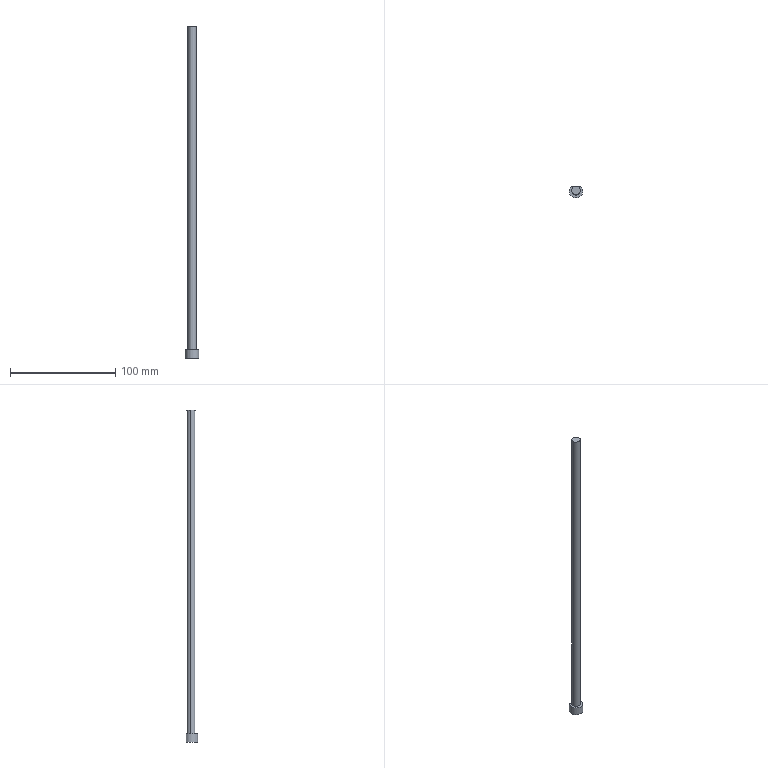Part | Creo | 1 solid | 7 faces | box 13 x 11 x 315 mm | volume 16390 mm3 | plane 4 | cylinder 3 | commonest cylinder face diameters 8 x2 13 x1
STEP:
#1=CARTESIAN_POINT('',(0.,0.,0.));
#2=DIRECTION('',(0.,0.,1.));
#3=DIRECTION('',(1.,0.,0.));
#4=AXIS2_PLACEMENT_3D('',#1,#2,#3);
#5=CARTESIAN_POINT('',(-35.209,-218.32,-330.441));
#6=VERTEX_POINT('',#5);
#7=CARTESIAN_POINT('',(-44.59,-218.32,-330.441));
#8=VERTEX_POINT('',#7);
#9=CARTESIAN_POINT('',(-35.209,-218.32,-330.441));
#10=DIRECTION('',(-1.,0.,0.));
#11=VECTOR('',#10,9.381);
#12=LINE('',#9,#11);
#13=EDGE_CURVE('',#6,#8,#12,.T.);
#14=ORIENTED_EDGE('',*,*,#13,.F.);
#15=CARTESIAN_POINT('',(-39.899,-222.82,-330.441));
#16=DIRECTION('',(0.,0.,-1.));
#17=DIRECTION('',(0.7216,0.6923,0.));
#18=AXIS2_PLACEMENT_3D('',#15,#16,#17);
#19=CIRCLE('',#18,6.5);
#20=EDGE_CURVE('',#6,#8,#19,.T.);
#21=ORIENTED_EDGE('',*,*,#20,.T.);
#22=EDGE_LOOP('',(#14,#21));
#23=FACE_OUTER_BOUND('',#22,.F.);
#24=CARTESIAN_POINT('',(-43.899,-222.82,-330.441));
#25=VERTEX_POINT('',#24);
#26=CARTESIAN_POINT('',(-35.899,-222.82,-330.441));
#27=VERTEX_POINT('',#26);
#28=CARTESIAN_POINT('',(-39.899,-222.82,-330.441));
#29=DIRECTION('',(0.,0.,-1.));
#30=DIRECTION('',(-1.,0.,0.));
#31=AXIS2_PLACEMENT_3D('',#28,#29,#30);
#32=CIRCLE('',#31,4.);
#33=EDGE_CURVE('',#25,#27,#32,.T.);
#34=ORIENTED_EDGE('',*,*,#33,.F.);
#35=CARTESIAN_POINT('',(-39.899,-222.82,-330.441));
#36=DIRECTION('',(0.,0.,-1.));
#37=DIRECTION('',(1.,0.,0.));
#38=AXIS2_PLACEMENT_3D('',#35,#36,#37);
#39=CIRCLE('',#38,4.);
#40=EDGE_CURVE('',#27,#25,#39,.T.);
#41=ORIENTED_EDGE('',*,*,#40,.F.);
#42=EDGE_LOOP('',(#34,#41));
#43=FACE_BOUND('',#42,.F.);
#44=CARTESIAN_POINT('',(-39.899,-222.82,-330.441));
#45=DIRECTION('',(0.,0.,-1.));
#46=DIRECTION('',(-1.,0.,0.));
#47=AXIS2_PLACEMENT_3D('',#44,#45,#46);
#48=PLANE('',#47);
#49=ADVANCED_FACE('',(#23,#43),#48,.F.);
#50=CARTESIAN_POINT('',(-35.899,-222.82,-23.441));
#51=VERTEX_POINT('',#50);
#52=CARTESIAN_POINT('',(-43.899,-222.82,-23.441));
#53=VERTEX_POINT('',#52);
#54=CARTESIAN_POINT('',(-39.899,-222.82,-23.441));
#55=DIRECTION('',(0.,0.,1.));
#56=DIRECTION('',(1.,0.,0.));
#57=AXIS2_PLACEMENT_3D('',#54,#55,#56);
#58=CIRCLE('',#57,4.);
#59=EDGE_CURVE('',#51,#53,#58,.T.);
#60=ORIENTED_EDGE('',*,*,#59,.T.);
#61=CARTESIAN_POINT('',(-43.899,-222.82,-330.441));
#62=DIRECTION('',(0.,0.,1.));
#63=VECTOR('',#62,307.);
#64=LINE('',#61,#63);
#65=EDGE_CURVE('',#25,#53,#64,.T.);
#66=ORIENTED_EDGE('',*,*,#65,.F.);
#67=ORIENTED_EDGE('',*,*,#33,.T.);
#68=CARTESIAN_POINT('',(-35.899,-222.82,-330.441));
#69=DIRECTION('',(0.,0.,1.));
#70=VECTOR('',#69,307.);
#71=LINE('',#68,#70);
#72=EDGE_CURVE('',#27,#51,#71,.T.);
#73=ORIENTED_EDGE('',*,*,#72,.T.);
#74=EDGE_LOOP('',(#60,#66,#67,#73));
#75=FACE_OUTER_BOUND('',#74,.F.);
#76=CARTESIAN_POINT('',(-39.899,-222.82,-653.441));
#77=DIRECTION('',(0.,0.,1.));
#78=DIRECTION('',(1.,0.,0.));
#79=AXIS2_PLACEMENT_3D('',#76,#77,#78);
#80=CYLINDRICAL_SURFACE('',#79,4.);
#81=ADVANCED_FACE('',(#75),#80,.T.);
#82=CARTESIAN_POINT('',(-39.899,-222.82,-23.441));
#83=DIRECTION('',(0.,0.,1.));
#84=DIRECTION('',(-1.,0.,0.));
#85=AXIS2_PLACEMENT_3D('',#82,#83,#84);
#86=CIRCLE('',#85,4.);
#87=EDGE_CURVE('',#53,#51,#86,.T.);
#88=ORIENTED_EDGE('',*,*,#87,.F.);
#89=ORIENTED_EDGE('',*,*,#59,.F.);
#90=EDGE_LOOP('',(#88,#89));
#91=FACE_OUTER_BOUND('',#90,.F.);
#92=CARTESIAN_POINT('',(-39.899,-222.82,-23.441));
#93=DIRECTION('',(0.,0.,-1.));
#94=DIRECTION('',(-1.,0.,0.));
#95=AXIS2_PLACEMENT_3D('',#92,#93,#94);
#96=PLANE('',#95);
#97=ADVANCED_FACE('',(#91),#96,.F.);
#98=ORIENTED_EDGE('',*,*,#87,.T.);
#99=ORIENTED_EDGE('',*,*,#72,.F.);
#100=ORIENTED_EDGE('',*,*,#40,.T.);
#101=ORIENTED_EDGE('',*,*,#65,.T.);
#102=EDGE_LOOP('',(#98,#99,#100,#101));
#103=FACE_OUTER_BOUND('',#102,.F.);
#104=CARTESIAN_POINT('',(-39.899,-222.82,-653.441));
#105=DIRECTION('',(0.,0.,1.));
#106=DIRECTION('',(1.,0.,0.));
#107=AXIS2_PLACEMENT_3D('',#104,#105,#106);
#108=CYLINDRICAL_SURFACE('',#107,4.);
#109=ADVANCED_FACE('',(#103),#108,.T.);
#110=CARTESIAN_POINT('',(-44.59,-218.32,-338.441));
#111=VERTEX_POINT('',#110);
#112=CARTESIAN_POINT('',(-44.59,-218.32,-330.441));
#113=DIRECTION('',(0.,0.,-1.));
#114=VECTOR('',#113,8.);
#115=LINE('',#112,#114);
#116=EDGE_CURVE('',#8,#111,#115,.T.);
#117=ORIENTED_EDGE('',*,*,#116,.T.);
#118=CARTESIAN_POINT('',(-35.209,-218.32,-338.441));
#119=VERTEX_POINT('',#118);
#120=CARTESIAN_POINT('',(-35.209,-218.32,-338.441));
#121=DIRECTION('',(-1.,0.,0.));
#122=VECTOR('',#121,9.381);
#123=LINE('',#120,#122);
#124=EDGE_CURVE('',#119,#111,#123,.T.);
#125=ORIENTED_EDGE('',*,*,#124,.F.);
#126=CARTESIAN_POINT('',(-35.209,-218.32,-338.441));
#127=DIRECTION('',(0.,0.,1.));
#128=VECTOR('',#127,8.);
#129=LINE('',#126,#128);
#130=EDGE_CURVE('',#119,#6,#129,.T.);
#131=ORIENTED_EDGE('',*,*,#130,.T.);
#132=ORIENTED_EDGE('',*,*,#13,.T.);
#133=EDGE_LOOP('',(#117,#125,#131,#132));
#134=FACE_OUTER_BOUND('',#133,.F.);
#135=CARTESIAN_POINT('',(-39.899,-218.32,-338.441));
#136=DIRECTION('',(0.,1.,0.));
#137=DIRECTION('',(0.,0.,1.));
#138=AXIS2_PLACEMENT_3D('',#135,#136,#137);
#139=PLANE('',#138);
#140=ADVANCED_FACE('',(#134),#139,.T.);
#141=CARTESIAN_POINT('',(-39.899,-222.82,-338.441));
#142=DIRECTION('',(0.,0.,1.));
#143=DIRECTION('',(-0.7216,0.6923,0.));
#144=AXIS2_PLACEMENT_3D('',#141,#142,#143);
#145=CIRCLE('',#144,6.5);
#146=EDGE_CURVE('',#111,#119,#145,.T.);
#147=ORIENTED_EDGE('',*,*,#146,.F.);
#148=ORIENTED_EDGE('',*,*,#116,.F.);
#149=ORIENTED_EDGE('',*,*,#20,.F.);
#150=ORIENTED_EDGE('',*,*,#130,.F.);
#151=EDGE_LOOP('',(#147,#148,#149,#150));
#152=FACE_OUTER_BOUND('',#151,.F.);
#153=CARTESIAN_POINT('',(-39.899,-222.82,-330.441));
#154=DIRECTION('',(0.,0.,-1.));
#155=DIRECTION('',(-1.,0.,0.));
#156=AXIS2_PLACEMENT_3D('',#153,#154,#155);
#157=CYLINDRICAL_SURFACE('',#156,6.5);
#158=ADVANCED_FACE('',(#152),#157,.T.);
#159=ORIENTED_EDGE('',*,*,#146,.T.);
#160=ORIENTED_EDGE('',*,*,#124,.T.);
#161=EDGE_LOOP('',(#159,#160));
#162=FACE_OUTER_BOUND('',#161,.F.);
#163=CARTESIAN_POINT('',(71.601,-77.127,-338.441));
#164=DIRECTION('',(0.,0.,-1.));
#165=DIRECTION('',(-1.,0.,0.));
#166=AXIS2_PLACEMENT_3D('',#163,#164,#165);
#167=PLANE('',#166);
#168=ADVANCED_FACE('',(#162),#167,.T.);
#169=CLOSED_SHELL('',(#49,#81,#97,#109,#140,#158,#168));
#170=MANIFOLD_SOLID_BREP('',#169);
#171=(LENGTH_UNIT()NAMED_UNIT(*)SI_UNIT(.MILLI.,.METRE.));
#172=UNCERTAINTY_MEASURE_WITH_UNIT(LENGTH_MEASURE(0.03154),#171,'','');
#173=(NAMED_UNIT(*)PLANE_ANGLE_UNIT()SI_UNIT($,.RADIAN.));
#174=PLANE_ANGLE_MEASURE_WITH_UNIT(PLANE_ANGLE_MEASURE(0.01745),#173);
#175=(CONVERSION_BASED_UNIT('DEGREE',#174)NAMED_UNIT(*)PLANE_ANGLE_UNIT());
#176=(NAMED_UNIT(*)SI_UNIT($,.STERADIAN.)SOLID_ANGLE_UNIT());
#177=(GEOMETRIC_REPRESENTATION_CONTEXT(3)GLOBAL_UNCERTAINTY_ASSIGNED_CONTEXT((#172))GLOBAL_UNIT_ASSIGNED_CONTEXT((#171,#175,#176))REPRESENTATION_CONTEXT('',''));
#178=ADVANCED_BREP_SHAPE_REPRESENTATION('',(#4,#170),#177);